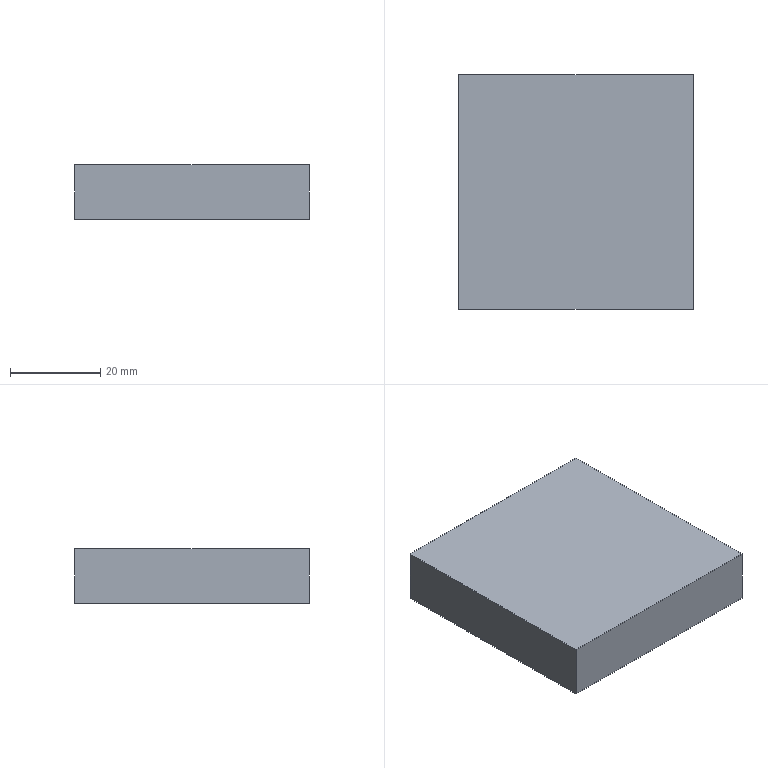NC program | NX | posted with a generic post | part box 52 x 52 x 12 mm
Lines 19 to 849 of 2608:
(ADAPTIVE_MILLING , TOOL : D4-12-D4-50-3T--FINISH)
N36 T02 M6
N38 G53
N40 G17 G0 G90 X-33.203 Y-2.883 S6500 M3
N42 G43 Z30.15 H2
N44 Z-4.
N46 G94 G1 X-33.069 Y-2.816 Z-4.937 F2500.
N48 X-32.935 Y-2.748 Z-5.308
N50 X-32.8 Y-2.681 Z-5.58
N52 X-32.666 Y-2.614 Z-5.8
N54 X-32.532 Y-2.547 Z-5.984
N56 X-32.398 Y-2.479 Z-6.142
N58 X-32.264 Y-2.412 Z-6.28
N60 X-32.13 Y-2.345 Z-6.4
N62 X-31.996 Y-2.278 Z-6.505
N64 X-31.862 Y-2.21 Z-6.598
N66 X-31.728 Y-2.143 Z-6.679
N68 X-31.594 Y-2.076 Z-6.75
N70 X-31.46 Y-2.009 Z-6.81
N72 X-31.325 Y-1.942 Z-6.862
N74 X-31.191 Y-1.874 Z-6.905
N76 X-31.057 Y-1.807 Z-6.939
N78 X-30.923 Y-1.74 Z-6.966
N80 X-30.789 Y-1.673 Z-6.985
N82 X-30.655 Y-1.605 Z-6.996
N84 X-30.521 Y-1.538 Z-7.
N86 G3 X-29.614 Y-1.063 R20.387
N88 X-29.254 Y0.029 R2.109
N90 X-29.102 Y4.194 R37.621
N92 G1 X-29.098 Y6.69
N94 X-29.096 Y26.39
N96 G2 X-27.893 Y28.24 R2.328
N98 X-25.32 Y28.976 R5.942
N100 X-19.923 Y29.099 R65.543
N102 G1 X26.36 Y29.097
N104 G2 X28.249 Y27.874 R2.325
N106 X28.992 Y25.148 R6.224
N108 X29.1 Y19.951 R72.546
N110 G1 Y-26.307
N112 G2 X27.919 Y-28.22 R2.297
N114 X25.299 Y-28.974 R5.956
N116 X19.952 Y-29.096 R65.663
N118 G1 X-26.311 Y-29.097
N120 G2 X-28.196 Y-27.957 R2.28
N122 X-28.968 Y-25.396 R5.753
N124 X-29.099 Y-19.949 R62.096
N126 G1 Y-2.449
N128 G2 X-28.85 Y0.18 R43.276
N130 G3 X-28.699 Y6.94 R88.157
N132 G1 X-28.694 Y25.29
N134 G2 X-26.925 Y27.842 R3.092
N136 X-23.837 Y28.591 R7.911
N138 X-17.239 Y28.699 R101.51
N140 G1 X25.186 Y28.696
N142 G2 X27.795 Y27.011 R3.06
N144 X28.579 Y23.984 R7.511
N146 X28.7 Y17.587 R88.534
N148 G1 Y-25.184
N150 G2 X27.02 Y-27.787 R3.054
N152 X23.99 Y-28.574 R7.481
N154 X18.593 Y-28.696 R72.904
N156 G1 X-25.137
N158 G2 X-27.79 Y-27.016 R3.047
N160 X-28.577 Y-23.988 R7.485
N162 X-28.699 Y-17.591 R87.654
N164 G1 X-28.697 Y-3.26
N166 G2 X-28.423 Y0.687 R89.536
N168 G3 X-28.299 Y7.39 R124.447
N170 G1 X-28.296 Y24.19
N172 G2 X-26.201 Y27.412 R3.556
N174 X-22.959 Y28.18 R8.772
N176 X-16.111 Y28.299 R101.445
N178 G1 X24.186 Y28.295
N180 G2 X27.432 Y26.163 R3.573
N182 X28.18 Y22.962 R8.864
N184 X28.3 Y17.265 R83.095
N186 G1 Y-24.085
N188 G2 X26.157 Y-27.431 R3.579
N190 X22.956 Y-28.177 R8.881
N192 X16.009 Y-28.296 R104.217
N194 G1 X-24.187 Y-28.295
N196 G2 X-27.411 Y-26.2 R3.559
N198 X-28.18 Y-22.955 R8.771
N200 X-28.299 Y-16.007 R104.053
N202 G1 X-28.298 Y-4.16
N204 G2 X-28.023 Y0.824 R93.452
N206 G3 X-27.899 Y7.54 R143.415
N208 G1 X-27.896 Y23.29
N210 G2 X-25.446 Y27.041 R3.95
N212 X-21.994 Y27.787 R10.026
N214 X-14.647 Y27.899 R121.769
N216 G1 X23.303 Y27.894
N218 G2 X27.027 Y25.477 R3.938
N220 X27.781 Y22.078 R9.803
N222 X27.899 Y16.281 R89.768
N224 G1 X27.9 Y-23.119
N226 G2 X25.417 Y-27.052 R3.982
N228 X22.062 Y-27.779 R9.961
N230 X14.964 Y-27.896 R112.386
N232 G1 X-23.287 Y-27.894
N234 G2 X-27.042 Y-25.442 R3.955
N236 X-27.779 Y-22.09 R9.886
N238 X-27.899 Y-16.242 R89.274
N240 X-27.873 Y-3.411 R887.241
N242 G3 X-27.546 Y3.077 R283.175
N244 X-27.499 Y8.24 R556.812
N246 G1 X-27.496 Y22.44
N248 G2 X-26.384 Y25.558 R4.314
N250 X-23.3 Y27.114 R5.847
N252 X-18.821 Y27.478 R24.54
N254 G1 X-14.171 Y27.499
N256 X22.429 Y27.495
N258 G2 X25.476 Y26.458 R4.336
N260 X27.079 Y23.454 R5.64
N262 X27.474 Y19.08 R22.258
N264 G1 X27.5 Y14.13
N266 X27.498 Y-22.42
N268 G2 X26.463 Y-25.471 R4.34
N270 X23.408 Y-27.087 R5.688
N272 X18.982 Y-27.472 R23.016
N274 G1 X14.033 Y-27.496
N276 X-22.417 Y-27.494
N278 G2 X-25.437 Y-26.493 R4.362
N280 X-27.067 Y-23.503 R5.58
N282 X-27.469 Y-19.28 R21.175
N284 X-27.465 Y-3.531 R681.297
N286 G3 X-27.139 Y3.621 R281.267
N288 G1 X-27.099 Y9.09
N290 X-27.083 Y22.14
N292 G2 X-24.31 Y26.193 R4.426
N294 X-20.661 Y26.974 R10.996
N296 X-14.663 Y27.098 R93.785
N298 G1 X21.387 Y27.096
N300 G2 X23.887 Y26.711 R6.038
N302 X26.361 Y23.897 R4.72
N304 X27.013 Y20.066 R13.222
N306 X27.1 Y13.017 R161.291
N308 G1 X27.098 Y-21.633
N310 G2 X26.435 Y-24.414 R5.075
N312 X23.56 Y-26.474 R5.081
N314 X19.51 Y-27.035 R15.777
N316 X12.81 Y-27.096 R243.584
N318 G1 X-21.59 Y-27.095
N320 G2 X-24.292 Y-26.507 R5.234
N322 X-26.446 Y-23.653 R4.972
N324 X-27.025 Y-19.807 R14.666
N326 X-27.099 Y-12.808 R193.167
N328 X-27.047 Y-3.309 R326.95
N330 G3 X-26.699 Y9.04 R192.271
N332 G2 X-26.676 Y21.59 R848.175
N334 X-23.752 Y25.786 R4.613
N336 X-19.902 Y26.58 R11.694
N338 X-12.404 Y26.698 R126.405
N340 G1 X20.946 Y26.694
N342 G2 X23.751 Y26.099 R5.624
N344 X26.002 Y23.197 R5.089
N346 X26.621 Y19.207 R14.742
N348 X26.699 Y12.358 R180.282
N350 G1 X26.697 Y-20.942
N352 G2 X26.127 Y-23.703 R5.658
N354 X23.191 Y-26.001 R5.073
N356 X19.201 Y-26.618 R14.824
N358 X12.352 Y-26.696 R181.384
N360 G1 X-20.948 Y-26.693
N362 G2 X-23.754 Y-26.097 R5.622
N364 X-26.004 Y-23.188 R5.086
N366 X-26.621 Y-19.199 R14.827
N368 X-26.698 Y-12.35 R181.102
N370 X-26.625 Y-2.951 R252.379
N372 G3 X-26.299 Y8.99 R188.646
N374 G2 X-26.276 Y20.94 R861.9
N376 X-23.218 Y25.378 R4.788
N378 X-19.467 Y26.164 R11.824
N380 X-13.369 Y26.297 R92.954
N382 G1 X19.981 Y26.296
N384 G2 X22.691 Y25.939 R7.518
N386 X25.447 Y23.053 R4.901
N388 X26.188 Y19.139 R12.831
N390 X26.299 Y11.691 R136.173
N392 G1 X26.297 Y-20.209
N394 G2 X25.813 Y-22.993 R6.451
N396 X22.923 Y-25.495 R5.036
N398 X18.95 Y-26.196 R13.634
N400 X11.701 Y-26.296 R148.157
N402 G1 X-20.249 Y-26.293
N404 G2 X-22.984 Y-25.816 R6.423
N406 X-25.526 Y-22.841 R5.064
N408 X-26.204 Y-18.861 R14.027
N410 X-26.298 Y-11.712 R153.865
N412 X-26.213 Y-2.814 R219.865
N414 G3 X-25.899 Y10.24 R207.979
N416 G2 X-25.873 Y20.39 R545.707
N418 X-22.664 Y24.987 R4.933
N420 X-18.66 Y25.778 R12.698
N422 X-11.012 Y25.898 R132.132
N424 G1 X19.588 Y25.894
N426 G2 X22.383 Y25.449 R7.065
N428 X25.078 Y22.436 R5.109
N430 X25.798 Y18.364 R13.92
N432 X25.899 Y10.966 R151.238
N434 G1 X25.897 Y-19.534
N436 G2 X25.491 Y-22.287 R7.316
N438 X22.524 Y-25.04 R5.057
N440 X18.556 Y-25.782 R13.285
N442 X11.008 Y-25.895 R137.136
N444 G1 X-19.542 Y-25.894
N446 G2 X-22.294 Y-25.486 R7.319
N448 X-25.043 Y-22.522 R5.055
N450 X-25.785 Y-18.553 R13.286
N452 X-25.898 Y-11.005 R137.233
N454 X-25.619 Y1.446 R194.549
N456 G3 X-25.499 Y10.19 R261.34
N458 G2 X-25.47 Y19.84 R456.122
N460 X-24.039 Y23.366 R5.121
N462 X-20.63 Y25.047 R6.763
N464 X-15.856 Y25.467 R26.018
N466 G1 X-10.306 Y25.498
N468 X18.944 Y25.493
N470 G2 X21.75 Y25.096 R7.795
N472 X24.605 Y22.1 R5.129
N474 X25.378 Y18.091 R13.194
N476 X25.499 Y10.243 R135.704
N478 G1 X25.497 Y-18.907
N480 G2 X25.093 Y-21.761 R7.81
N482 X22.157 Y-24.578 R5.112
N484 X18.251 Y-25.362 R12.789
N486 X10.254 Y-25.495 R128.624
N488 G1 X-18.946 Y-25.493
N490 G2 X-21.752 Y-25.096 R7.758
N492 X-24.584 Y-22.149 R5.106
N494 X-25.373 Y-18.143 R13.004
N496 X-25.498 Y-10.245 R132.531
N498 X-25.212 Y1.693 R211.686
N500 G3 X-25.099 Y10.44 R286.906
N502 G2 X-25.069 Y19.29 R390.549
N504 X-23.818 Y22.7 R5.337
N506 X-20.585 Y24.532 R6.353
N508 X-15.924 Y25.05 R21.484
N510 X-9.524 Y25.097 R446.678
N512 G1 X18.276 Y25.094
N514 G2 X21.139 Y24.734 R8.683
N516 X24.178 Y21.656 R5.191
N518 X24.968 Y17.65 R13.19
N520 X25.099 Y9.503 R135.711
N522 G1 X25.098 Y-17.997
N524 G2 X24.835 Y-20.826 R10.511
N526 X21.816 Y-24.108 R5.098
N528 X17.771 Y-24.955 R12.586
N530 X11.124 Y-25.094 R101.349
N532 G1 X-17.976 Y-25.095
N534 G2 X-20.853 Y-24.825 R10.55
N536 X-24.118 Y-21.798 R5.098
N538 X-24.956 Y-17.804 R12.576
N540 X-25.097 Y-11.157 R99.932
N542 X-24.815 Y1.692 R226.264
N544 G3 X-24.699 Y10.44 R296.88
N546 G2 X-24.667 Y18.79 R318.957
N548 X-23.408 Y22.243 R5.481
N550 X-20.104 Y24.124 R6.465
N552 X-15.543 Y24.644 R21.288
N554 X-9.343 Y24.697 R350.214
N556 G1 X17.707 Y24.693
N558 G2 X20.622 Y24.34 R9.17
N560 X23.738 Y21.258 R5.242
N562 X24.556 Y17.257 R12.987
N564 X24.697 Y10.91 R96.9
N566 G1 X24.699 Y-16.89
N568 G2 X24.508 Y-20.028 R15.227
N570 X21.373 Y-23.685 R5.152
N572 X17.333 Y-24.547 R12.6
N574 X10.936 Y-24.694 R93.256
N576 G1 X-17.364
N578 G2 X-20.342 Y-24.426 R11.256
N580 X-23.698 Y-21.348 R5.175
N582 X-24.552 Y-17.303 R12.7
N584 X-24.696 Y-10.906 R94.987
N586 X-24.42 Y1.591 R230.578
N588 G3 X-24.299 Y16.29 R462.447
N590 G2 X-24.128 Y19.43 R16.999
N592 X-20.931 Y23.271 R5.218
N594 X-16.992 Y24.134 R12.439
N596 X-10.146 Y24.296 R92.068
N598 G1 X16.754 Y24.295
N600 G2 X19.737 Y24.056 R12.555
N602 X23.279 Y20.909 R5.244
N604 X24.149 Y16.82 R12.758
N606 X24.297 Y10.173 R97.407
N608 G1 X24.298 Y-16.827
N610 G2 X24.04 Y-19.807 R11.865
N612 X20.976 Y-23.247 R5.222
N614 X17.091 Y-24.122 R12.225
N616 X10.095 Y-24.294 R89.484
N618 G1 X-16.755
N620 G2 X-19.738 Y-24.055 R12.487
N622 X-23.281 Y-20.902 R5.242
N624 X-24.144 Y-16.862 R12.722
N626 X-24.297 Y-9.515 R105.066
N628 X-24.017 Y1.739 R248.67
N630 G3 X-23.896 Y16.69 R507.635
N632 G2 X-23.525 Y19.704 R9.597
N634 X-20.419 Y22.886 R5.363
N636 X-16.225 Y23.753 R13.229
N638 X-9.378 Y23.896 R104.908
N640 G1 X16.222 Y23.895
N642 G2 X19.304 Y23.642 R12.696
N644 X22.882 Y20.423 R5.327
N646 X23.742 Y16.382 R12.915
N648 X23.897 Y9.885 R92.481
N650 G1 X23.898 Y-15.765
N652 G2 X23.713 Y-19.004 R16.843
N654 X20.508 Y-22.843 R5.283
N656 X16.371 Y-23.739 R12.784
N658 X9.474 Y-23.894 R98.26
N660 G1 X-16.226
N662 G2 X-19.307 Y-23.64 R12.618
N664 X-22.844 Y-20.507 R5.296
N666 X-23.737 Y-16.421 R12.662
N668 X-23.896 Y-8.775 R105.551
N670 X-23.615 Y1.888 R283.895
N672 G3 X-23.494 Y16.34 R517.881
N674 G2 X-23.084 Y19.348 R9.137
N676 X-19.904 Y22.504 R5.465
N678 X-15.708 Y23.353 R13.598
N680 X-9.111 Y23.496 R102.82
N682 G1 X15.139 Y23.495
N684 G2 X18.431 Y23.328 R18.939
N686 X22.463 Y20. R5.374
N688 X23.338 Y15.911 R13.
N690 X23.497 Y9.065 R96.07
N692 G1 X23.498 Y-15.685
N694 G2 X23.257 Y-18.769 R13.41
N696 X20.086 Y-22.422 R5.346
N698 X16.104 Y-23.318 R12.507
N700 X9.058 Y-23.493 R90.027
N702 G1 X-15.692 Y-23.494
N704 G2 X-18.775 Y-23.253 R13.369
N706 X-22.464 Y-19.993 R5.379
N708 X-23.338 Y-15.903 R13.045
N710 X-23.492 Y-7.957 R108.224
N712 X-23.201 Y2.434 R383.109
N714 G3 X-23.09 Y16.04 R538.211
N716 G2 X-22.607 Y19.084 R8.454
N718 X-19.383 Y22.127 R5.569
N720 X-15.181 Y22.955 R14.02
N722 X-8.334 Y23.096 R108.075
N724 G1 X-1.331
N726 X-0.967 Y23.13
N728 X7.336 Y23.096
N730 G2 X16.736 Y23.062 R390.242
N732 X20.049 Y22.088 R6.251
N734 X22.338 Y18.797 R6.155
N736 X23.005 Y14.359 R17.563
N738 X23.098 Y7.161 R175.859
N740 G1 Y1.31
N742 X23.13 Y0.967
N744 X23.098 Y-6.134
N746 G2 X23.072 Y-16.584 R532.456
N748 X22.253 Y-19.794 R6.607
N750 X18.97 Y-22.278 R5.948
N752 X14.541 Y-22.992 R16.633
N754 X7.142 Y-23.094 R161.807
N756 G1 X1.351
N758 X0.967 Y-23.13
N760 X-7.388 Y-23.094
N762 G2 X-16.737 Y-23.061 R385.352
N764 X-20.091 Y-22.058 R6.214
N766 X-22.33 Y-18.816 R6.156
N768 X-23.008 Y-14.279 R17.746
N770 X-22.976 Y-2.622 R166.389
N772 G1 X-23.13 Y-0.968
N774 X-23.109 Y1.372
N776 G3 X-22.711 Y8.152 R48.09
N778 G2 X-22.669 Y16.19 R466.644
N780 X-21.772 Y19.479 R6.536
N782 X-18.465 Y21.895 R6.09
N784 X-14.083 Y22.592 R16.898
N786 X-4.46 Y22.696 R215.816
N788 G1 X-3.297 Y22.914
N790 X-0.967 Y23.13
N792 X1.372 Y23.109
N794 G3 X5.483 Y22.73 R48.67
N796 X15.687 Y22.683 R856.326
N798 G2 X18.816 Y22.123 R8.025
N800 X21.758 Y18.842 R5.702
N802 X22.569 Y14.482 R14.855
N804 X22.698 Y6.735 R135.878
N806 G1 X22.699 Y4.393
N808 X22.914 Y3.297
N810 X23.098 Y1.306
N812 G3 X23.686 Y0.99 R0.4
N814 X23.898 Y1.274 Z-6.954 R0.457
N816 G1 X24.046 Y1.669 Z-6.9
N818 X24.338 Y2.459 F15000.
N820 X24.349 Y2.556
N822 G3 X24.269 Y6.875 R118.157
N824 G1 X24.18 Y8.444
N826 X23.691 Y15.466
N828 G3 X23.172 Y18.443 R19.592
N830 X22.521 Y20.022 R8.255
N832 X21.376 Y21.845 R13.475
N834 X20.412 Y22.662 R3.75
N836 X18.87 Y23.411 R10.132
N838 X17.68 Y23.687 R5.194
N840 X15.235 Y23.869 R25.898
N842 G1 X4.895 Y24.101
N844 X4.792 Y24.075
N846 X4.07 Y23.788
N848 X3.577 Y23.588 Z-6.968 F2500.
N850 G3 X3.413 Y23.399 Z-7. R0.427
N852 X3.698 Y22.853 R0.4
N854 X6.538 Y22.374 R16.722
N856 X14.736 Y22.291 R203.781
N858 G2 X17.852 Y21.918 R10.478
N860 X21.263 Y18.62 R5.577
N862 X22.133 Y14.479 R13.536
N864 X22.297 Y7.582 R97.345
N866 G1 X22.305 Y6.116
N868 G2 X22.704 Y4.367 R12.651
N870 G3 X23.227 Y4.065 R0.4
N872 X23.496 Y4.363 Z-6.947 R0.442
N874 G1 X23.633 Y4.705 Z-6.9
N876 X23.945 Y5.497 F15000.
N878 X23.955 Y5.617
N880 X23.255 Y15.415
N882 G3 X21.855 Y20.065 R10.814
N884 X20.933 Y21.362 R10.211
N886 X19.718 Y22.33 R4.934
N888 X18.634 Y22.898 R8.608
N890 X17.218 Y23.276 R5.81
N892 X15.756 Y23.423 R11.855
N894 G1 X6.506 Y23.756
N896 X6.399 Y23.729
N898 X5.681 Y23.443
N900 X5.19 Y23.242 Z-6.968 F2500.
N902 G3 X5.026 Y23.052 Z-7. R0.426
N904 X5.311 Y22.507 R0.4
N906 G2 X6.816 Y22.13 R31.974
N908 G3 X10.403 Y21.908 R23.215
N910 G2 X15.587 Y21.842 R124.408
N912 X19.149 Y20.566 R6.05
N914 X21.203 Y17.201 R6.661
N916 X21.822 Y12.502 R20.252
N918 X21.904 Y7.439 R335.9
N920 G1 X22.311 Y6.099
N922 G3 X23.023 Y5.989 R0.4
N924 X23.1 Y6.301 Z-6.958 R0.571
N926 G1 X23.133 Y6.759 Z-6.9
N928 X23.195 Y7.631 F15000.
N930 X23.19 Y10.884
N932 G3 X22.882 Y14.73 R31.284
N934 G1 X22.751 Y15.662
N936 X22.597 Y16.589
N938 G3 X21.862 Y18.904 R11.251
N940 X20.749 Y20.623 R7.051
N942 G1 X20.378 Y21.047
N944 X19.989 Y21.456
N946 G3 X18.445 Y22.375 R4.558
N948 X15.592 Y23.006 R9.125
N950 G1 X7.664 Y23.475
N952 X7.573 Y23.467
N954 X7.484 Y23.443
N956 X6.788 Y23.147
N958 X6.32 Y22.941 Z-6.965 F2500.
N960 G3 X6.156 Y22.728 Z-7. R0.422
N962 X6.414 Y22.224 R0.4
N964 X10.005 Y21.552 R10.193
N966 G1 X14.895 Y21.457
N968 G2 X18.267 Y20.496 R6.631
N970 X20.697 Y17.091 R6.279
N972 X21.401 Y12.458 R18.018
N974 X21.5 Y8.528 R486.342
N976 X21.915 Y7.402 R9.311
N978 G3 X22.628 Y7.291 R0.4
N980 X22.705 Y7.604 Z-6.958 R0.571
N982 G1 X22.738 Y8.061 Z-6.9
N984 X22.8 Y8.933 F15000.
N986 X22.802 Y10.283
N988 X22.778 Y11.632
N990 G3 X22.538 Y14.07 R22.93
N992 G1 X22.387 Y15.065
N994 X22.21 Y16.055
N996 G3 X21.077 Y19.228 R12.198
N998 X19.873 Y20.75 R6.047
N1000 X16.523 Y22.437 R6.172
N1002 G1 X15.942 Y22.511
N1004 X12.399 Y22.815
N1006 X8.854 Y23.091
N1008 X8.759 Y23.084
N1010 X8.667 Y23.06
N1012 X7.977 Y22.764
N1014 X7.509 Y22.557 Z-6.965 F2500.
N1016 G3 X7.346 Y22.344 Z-7. R0.422
N1018 X7.604 Y21.841 R0.4
N1020 X9.009 Y21.381 R21.781
N1022 X12.664 Y21.112 R21.024
N1024 G2 X15.998 Y20.856 R16.752
N1026 X20.027 Y17.367 R5.661
N1028 X20.931 Y13.076 R13.84
N1030 X21.078 Y9.55 R88.608
N1032 G1 X21.515 Y8.479
N1034 G3 X22.148 Y8.333 R0.4
N1036 X22.289 Y8.673 Z-6.952 R0.449
N1038 G1 X22.323 Y9.078 Z-6.9
N1040 X22.399 Y10.01 F15000.
N1042 X22.363 Y11.088
N1044 X22.292 Y12.164
N1046 X22.094 Y13.796
N1048 X21.869 Y15.426
N1050 G3 X21.066 Y17.937 R8.806
N1052 X20.079 Y19.624 R10.342
N1054 X18.066 Y21.379 R6.442
N1056 X16.928 Y21.822 R5.677
N1058 X15.25 Y22.154 R9.051
N1060 X13.297 Y22.309 R23.886
N1062 G1 X9.924 Y22.427
N1064 X9.065 Y22.352
N1066 X8.773 Y22.33 Z-6.937 F2500.
N1068 X8.484 Y22.291 Z-6.975
N1070 X8.393 Y22.249 Z-6.987
N1072 X8.314 Y22.188 Z-7.
N1074 G3 X8.442 Y21.544 R0.4
N1076 X11.315 Y20.808 R6.799
N1078 G2 X14.695 Y20.607 R99.683
N1080 X19.634 Y16.912 R5.768
N1082 X20.531 Y12.62 R14.021
N1084 G1 X20.658 Y10.388
N1086 G2 X21.095 Y9.483 R7.797
N1088 G3 X21.727 Y9.336 R0.4
N1090 X21.869 Y9.677 Z-6.952 R0.449
N1092 G1 X21.904 Y10.081 Z-6.9
N1094 X21.979 Y11.015 F15000.
N1096 X21.919 Y11.746
N1098 X21.83 Y12.475
N1100 X21.466 Y14.805
N1102 G3 X20.257 Y18.363 R12.372
N1104 X19.229 Y19.713 R5.809
N1106 G1 X18.382 Y20.531
N1108 G3 X17.071 Y21.273 R4.196
N1110 X15.168 Y21.711 R7.605
N1112 G1 X12.984 Y21.903
N1114 X10.797 Y22.066
N1116 X9.888 Y21.991
N1118 X9.597 Y21.969 Z-6.937 F2500.
N1120 X9.307 Y21.929 Z-6.974
N1122 X9.217 Y21.887 Z-6.987
N1124 X9.138 Y21.826 Z-7.
N1126 G3 X9.266 Y21.182 R0.4
N1128 X12.138 Y20.417 R6.975
N1130 G2 X15.137 Y20.068 R21.809
N1132 X19.198 Y16.56 R5.758
N1134 X20.121 Y12.276 R13.709
N1136 G3 X20.239 Y10.99 R25.151
N1138 G1 X20.711 Y10.267
N1140 G3 X21.257 Y10.136 R0.4
N1142 X21.457 Y10.507 Z-6.944 R0.439
N1144 G1 X21.498 Y10.85 Z-6.9
N1146 X21.6 Y11.742 F15000.
N1148 X21.394 Y13.022
N1150 X21.158 Y14.296
N1152 G3 X20.378 Y16.892 R18.241
N1154 X19.157 Y18.887 R7.222
N1156 X18.322 Y19.779 R8.746
N1158 X15.888 Y21.074 R5.987
N1160 X14.303 Y21.384 R13.377
N1162 X11.629 Y21.687 R46.775
N1164 G1 X10.755 Y21.61
N1166 X10.464 Y21.588 Z-6.937 F2500.
N1168 X10.176 Y21.547 Z-6.974
N1170 X10.085 Y21.504 Z-6.987
N1172 X10.005 Y21.442 Z-7.
N1174 G3 X10.136 Y20.801 R0.4
N1176 G1 X10.935 Y20.399
N1178 G3 X13.445 Y19.928 R12.639
N1180 G2 X16.644 Y18.85 R7.158
N1182 X19.107 Y15.295 R6.539
N1184 X19.75 Y11.746 R19.683
N1186 G3 X19.903 Y11.27 R1.219
N1188 G1 X20.326 Y10.844
N1190 G3 X20.791 Y10.769 R0.401
N1192 X21.017 Y11.126 Z-6.944 R0.439
N1194 G1 X21.081 Y11.465 Z-6.9
N1196 X21.226 Y12.25 F15000.
N1198 X21.21 Y12.376
N1200 X20.091 Y16.139
N1202 G3 X18.77 Y18.463 R6.808
N1204 X17.749 Y19.516 R8.732
N1206 X15.836 Y20.566 R5.455
N1208 X13.947 Y21.082 R14.507
N1210 G1 X12.991 Y21.276
N1212 X12.033 Y21.46
N1214 X11.175 Y21.357
N1216 X10.667 Y21.287 Z-6.965 F2500.
N1218 G3 X10.452 Y21.128 Z-7. R0.422
N1220 X10.566 Y20.568 R0.4
N1222 X12.597 Y19.728 R4.65
N1224 G2 X15.324 Y18.978 R12.783
N1226 X18.516 Y15.414 R6.156
N1228 X19.273 Y12.226 R17.176
N1230 G3 X19.549 Y11.555 R1.142
N1232 G2 X19.919 Y11.255 R1.561
N1234 G3 X20.502 Y11.271 R0.4
N1236 X20.585 Y11.678 Z-6.945 R0.442
N1238 G1 X20.529 Y12.026 Z-6.9
N1240 G3 X20.004 Y14.74 R34.441 F15000.
N1242 X19.132 Y16.916 R8.469
N1244 G1 X18.529 Y17.943
N1246 G3 X17.483 Y19.071 R4.596
N1248 X15.174 Y20.322 R7.003
N1250 G1 X12.586 Y21.112
N1252 X12.47 Y21.113
N1254 X11.706 Y21.007
N1256 X11.447 Y20.974 Z-6.933 F2500.
N1258 X11.19 Y20.924 Z-6.967
N1260 G3 X10.99 Y20.763 Z-7. R0.414
N1262 X11.111 Y20.215 R0.4
N1264 X12.529 Y19.456 R3.178
N1266 G2 X15.095 Y18.545 R15.145
N1268 X18.168 Y14.859 R6.442
N1270 X18.838 Y12.395 R32.821
N1272 G3 X19.127 Y11.824 R1.217
N1274 G1 X19.591 Y11.529
N1276 G3 X20.081 Y11.576 R0.401
N1278 X20.196 Y11.985 Z-6.944 R0.438
N1280 G1 X20.159 Y12.325 Z-6.9
N1282 X20.063 Y13.191 F15000.
N1284 X19.04 Y16.004
N1286 G3 X17.319 Y18.412 R6.691
N1288 X15.125 Y19.872 R8.817
N1290 G1 X12.766 Y20.979
N1292 G3 X12.508 Y21.007 R0.417
N1294 G1 X11.871 Y20.863
N1296 X11.369 Y20.744 Z-6.966 F2500.
N1298 G3 X11.172 Y20.568 Z-7. R0.423
N1300 X11.235 Y20.095 R0.401
N1302 X12.868 Y19.041 R3.721
N1304 G2 X15.496 Y17.701 R10.382
N1306 X17.891 Y14.112 R7.188
N1308 G3 X18.519 Y12.286 R16.027
N1310 X18.963 Y11.928 R0.595
N1312 G1 X19.132 Y11.821
N1314 G3 X19.62 Y11.867 R0.401
N1316 X19.737 Y12.274 Z-6.944 R0.438
N1318 G1 X19.703 Y12.615 Z-6.9
N1320 X19.612 Y13.467 F15000.
N1322 X19.128 Y14.541
N1324 X18.626 Y15.608
N1326 G3 X17.47 Y17.38 R10.861
N1328 X16.565 Y18.41 R8.101
N1330 X14.621 Y19.624 R7.55
N1332 G1 X13.243 Y20.211
N1334 X12.371 Y20.345
N1336 X11.862 Y20.416 Z-6.966 F2500.
N1338 G3 X11.613 Y20.322 Z-7. R0.422
N1340 X11.584 Y19.737 R0.4
N1342 X13.197 Y18.566 R4.612
N1344 G2 X16.049 Y16.448 R8.512
N1346 X17.509 Y13.765 R9.087
N1348 G3 X18.209 Y12.26 R6.163
N1350 X18.792 Y11.99 R1.458
N1352 X19.282 Y12.182 R0.401
N1354 X19.255 Y12.608 Z-6.943 R0.437
N1356 G1 X19.107 Y12.914 Z-6.9
N1358 X18.824 Y13.495 F15000.
N1360 X13.27 Y19.941
N1362 G3 X12.999 Y20.078 R0.409
N1364 G1 X12.577 Y20.113
N1366 X12.319 Y20.137 Z-6.933 F2500.
N1368 X12.06 Y20.144 Z-6.966
N1370 G3 X11.827 Y20.025 Z-7. R0.412
N1372 X11.775 Y19.54 R0.401
N1374 X12.934 Y18.389 R3.179
N1376 G2 X15.34 Y16.491 R12.295
N1378 X17.11 Y13.559 R10.425
N1380 G3 X17.846 Y12.323 R3.999
N1382 X18.375 Y12.139 R10.106
N1384 X18.939 Y12.408 R0.44
N1386 X18.804 Y12.899 Z-6.931 R0.465
N1388 G1 X18.64 Y13.082 Z-6.9
N1390 X13.073 Y19.304 F15000.
N1392 X12.842 Y19.568 Z-6.945 F2500.
N1394 X12.599 Y19.821 Z-6.989
N1396 X12.529 Y19.866 Z-7.
N1398 G3 X11.958 Y19.242 R0.44
N1400 X13.084 Y17.94 R4.078
N1402 G2 X15.62 Y15.334 R11.856
N1404 X16.95 Y13.002 R45.794
N1406 G3 X17.552 Y12.32 R1.758
N1408 G1 X18.025 Y12.248
N1410 G3 X18.489 Y12.528 R0.441
N1412 X18.36 Y13.031 Z-6.93 R0.469
N1414 G1 X18.207 Y13.208 Z-6.9
N1416 X13.215 Y18.998 F15000.
N1418 X12.878 Y19.381 Z-6.965 F2500.
N1420 G3 X12.627 Y19.484 Z-7. R0.467
N1422 X12.219 Y18.815 R0.44
N1424 X13.231 Y17.42 R3.987
N1426 G2 X16.192 Y13.504 R16.018
N1428 G3 X17.094 Y12.384 R3.528
N1430 X17.644 Y12.294 R3.199
N1432 X18.105 Y12.567 R0.441
N1434 X17.991 Y13.065 Z-6.931 R0.465
N1436 G1 X17.836 Y13.253 Z-6.9
N1438 X13.302 Y18.74 F15000.
N1440 X13.152 Y18.926 Z-6.931 F2500.
N1442 X12.987 Y19.1 Z-6.961
N1444 G3 X12.702 Y19.19 Z-7. R0.449
N1446 X12.306 Y18.61 R0.44
N1448 X13.254 Y16.957 R4.289
N1450 G2 X15.865 Y13.294 R33.479
N1452 G3 X16.718 Y12.385 R2.96
N1454 X17.226 Y12.344 R2.284
N1456 X17.685 Y12.612 R0.441
N1458 X17.579 Y13.11 Z-6.931 R0.465
N1460 G1 X17.426 Y13.303 Z-6.9
N1462 X13.453 Y18.295 F15000.
N1464 X13.303 Y18.487 Z-6.931 F2500.
N1466 X13.14 Y18.668 Z-6.962
N1468 G3 X12.864 Y18.764 Z-7. R0.45
N1470 X12.45 Y18.184 R0.44
N1472 X13.446 Y16.191 R5.633
N1474 X15.538 Y13.124 R202.366
N1476 X16.332 Y12.378 R2.446
N1478 X16.88 Y12.353 R8.182
N1480 X17.294 Y12.634 R0.441
N1482 X17.189 Y13.119 Z-6.934 R0.47
N1484 G1 X17.03 Y13.328 Z-6.9
N1486 X13.54 Y17.926 F15000.
N1488 X13.413 Y18.097 Z-6.927 F2500.
N1490 X13.274 Y18.258 Z-6.954
N1492 G3 X12.939 Y18.358 Z-7. R0.444
N1494 X12.554 Y17.876 R0.44
N1496 X13.138 Y16.124 R3.678
N1498 X15.28 Y12.903 R22.977
N1500 X15.957 Y12.367 R1.569
N1502 G1 X16.449 Y12.357
N1504 G3 X16.862 Y12.636 R0.441
N1506 X16.763 Y13.118 Z-6.934 R0.471
N1508 G1 X16.605 Y13.334 Z-6.9
N1510 X13.587 Y17.467 F15000.
N1512 X13.463 Y17.64 Z-6.927 F2500.
N1514 X13.326 Y17.804 Z-6.955
N1516 G3 X12.995 Y17.912 Z-7. R0.444
N1518 X12.6 Y17.429 R0.44
N1520 X13.283 Y15.259 R4.752
N1522 X15.096 Y12.646 R10.935
N1524 X15.567 Y12.365 R0.928
N1526 G1 X16.017 Y12.361
N1528 G3 X16.429 Y12.637 R0.441
N1530 X16.336 Y13.118 Z-6.935 R0.474
N1532 G1 X16.179 Y13.339 Z-6.9
N1534 X13.635 Y16.941 F15000.
N1536 X13.515 Y17.115 Z-6.927 F2500.
N1538 X13.381 Y17.279 Z-6.954
N1540 G3 X13.048 Y17.391 Z-7. R0.444
N1542 X12.648 Y16.956 R0.44
N1544 X13.132 Y14.915 R3.865
N1546 X14.763 Y12.567 R7.722
N1548 X15.136 Y12.368 R0.816
N1550 G1 X15.586 Y12.364
N1552 G3 X15.998 Y12.639 R0.441
N1554 X15.915 Y13.11 Z-6.936 R0.47
N1556 G1 X15.756 Y13.344 Z-6.9
N1558 X13.631 Y16.48 F15000.
N1560 X13.514 Y16.657 Z-6.927 F2500.
N1562 X13.384 Y16.823 Z-6.954
N1564 G3 X13.053 Y16.941 Z-7. R0.444
N1566 X12.645 Y16.506 R0.44
N1568 X13.269 Y14.015 R4.248
N1570 X14.562 Y12.419 R4.435
N1572 X15.17 Y12.368 R1.686
N1574 X15.582 Y12.644 R0.441
N1576 X15.499 Y13.114 Z-6.936 R0.47
N1578 G1 X15.339 Y13.349 Z-6.9
N1580 X13.626 Y15.88 F15000.
N1582 X13.509 Y16.056 Z-6.927 F2500.
N1584 X13.379 Y16.223 Z-6.954
N1586 G3 X13.048 Y16.341 Z-7. R0.444
N1588 X12.639 Y15.906 R0.44
N1590 X13.388 Y13.261 R3.992
N1592 X14.221 Y12.4 R2.465
N1594 X14.727 Y12.372 R3.243
N1596 X15.14 Y12.65 R0.441
N1598 X15.055 Y13.118 Z-6.936 R0.471
N1600 G1 X14.894 Y13.355 Z-6.9
N1602 X13.62 Y15.231 F15000.
N1604 X13.503 Y15.407 Z-6.927 F2500.
N1606 X13.373 Y15.574 Z-6.954
N1608 G3 X13.041 Y15.691 Z-7. R0.444
N1610 X12.634 Y15.256 R0.44
N1612 X13.773 Y12.446 R3.258
N1614 X14.369 Y12.375 R1.219
N1616 X14.784 Y12.659 R0.441
N1618 X14.69 Y13.128 Z-6.936 R0.47
N1620 G1 X14.526 Y13.359 Z-6.9
N1622 X13.615 Y14.642 F15000.
N1624 X13.494 Y14.816 Z-6.927 F2500.
N1626 X13.361 Y14.98 Z-6.954
N1628 G3 X13.027 Y15.091 Z-7. R0.444
N1630 X12.628 Y14.656 R0.44
N1632 X13.41 Y12.485 R2.619
N1634 X14.006 Y12.378 R0.907
N1636 X14.424 Y12.668 R0.441
N1638 X14.318 Y13.142 Z-6.935 R0.475
N1640 G1 X14.155 Y13.364 Z-6.9
N1642 X13.611 Y14.102 F15000.
N1644 X13.487 Y14.273 Z-6.927 F2500.
N1646 X13.35 Y14.435 Z-6.954
N1648 G3 X13.015 Y14.54 Z-7. R0.444
N1650 X12.624 Y14.106 R0.44
N1652 X13.153 Y12.487 R1.98
N1654 X13.7 Y12.381 R0.817
N1656 X14.12 Y12.678 R0.441
N1658 X14.004 Y13.152 Z-6.935 R0.474
N1660 G1 X13.837 Y13.367 Z-6.9
N1662 X13.607 Y13.664 F15000.
N1664 X13.479 Y13.833 Z-6.927 F2500.
N1666 X13.338 Y13.991 Z-6.954
N1668 G3 X13.001 Y14.089 Z-7. R0.444
N1670 X12.62 Y13.656 R0.441
N1672 X12.949 Y12.5 R1.454
N1674 X13.412 Y12.383 R0.618
N1676 X13.753 Y13.106 R0.44
N1678 G1 X13.343 Y13.586
N1680 G3 X12.616 Y13.256 R0.44
N1682 X12.867 Y12.468 R0.867
N1684 X13.215 Y12.385 R1.399
N1686 X13.541 Y13.124 R0.44
N1688 G1 X13.325 Y13.349
N1690 G3 X12.614 Y13.006 R0.44